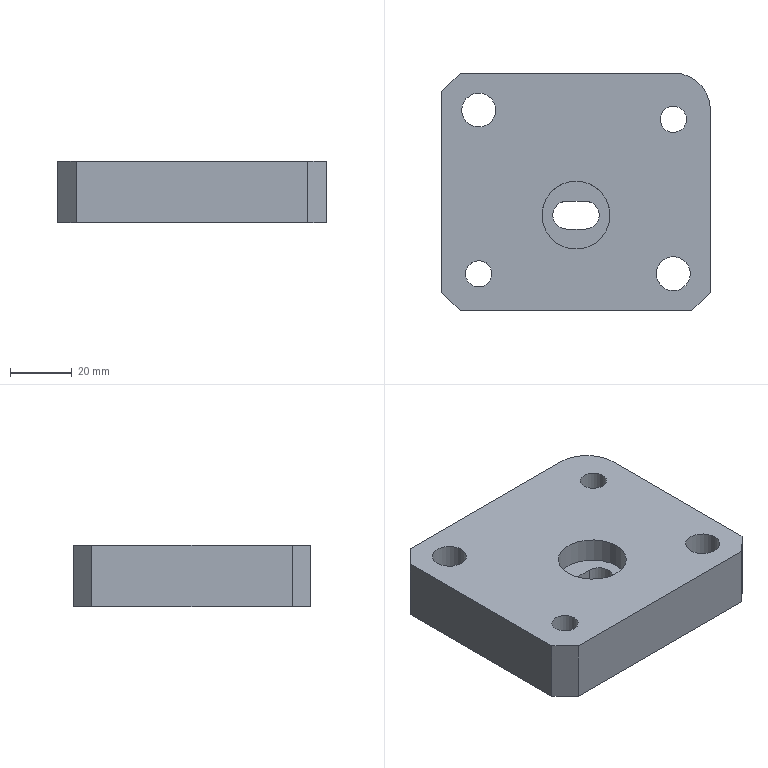Part | STEP file | lll_id3598_x_t | 1 solid | 28 faces | box 87 x 77 x 20 mm | volume 118043 mm3 | plane 16 | cylinder 12 | commonest cylinder face diameters 11 x4 8.5 x2 9.05 x2 17 x2 22 x1 24 x1
STEP:
#1=CARTESIAN_POINT('',(3550.234,-196.45,22.5));
#2=VERTEX_POINT('',#1);
#3=CARTESIAN_POINT('',(3555.734,-196.45,22.5));
#4=DIRECTION('',(0.,0.,-1.));
#5=DIRECTION('',(-1.,0.,0.));
#6=AXIS2_PLACEMENT_3D('',#3,#4,#5);
#7=CIRCLE('',#6,5.5);
#8=EDGE_CURVE('',#2,#2,#7,.T.);
#9=ORIENTED_EDGE('',*,*,#8,.T.);
#10=EDGE_LOOP('',(#9));
#11=FACE_BOUND('',#10,.T.);
#12=CARTESIAN_POINT('',(3543.734,-255.45,22.5));
#13=VERTEX_POINT('',#12);
#14=CARTESIAN_POINT('',(3543.734,-190.45,22.5));
#15=VERTEX_POINT('',#14);
#16=CARTESIAN_POINT('',(3543.734,-268.608,22.5));
#17=DIRECTION('',(0.,1.,0.));
#18=VECTOR('',#17,1.);
#19=LINE('',#16,#18);
#20=EDGE_CURVE('',#13,#15,#19,.T.);
#21=ORIENTED_EDGE('',*,*,#20,.F.);
#22=CARTESIAN_POINT('',(3549.734,-261.45,22.5));
#23=VERTEX_POINT('',#22);
#24=CARTESIAN_POINT('',(3727.771,-439.487,22.5));
#25=DIRECTION('',(0.7071,-0.7071,0.));
#26=VECTOR('',#25,1.);
#27=LINE('',#24,#26);
#28=EDGE_CURVE('',#13,#23,#27,.T.);
#29=ORIENTED_EDGE('',*,*,#28,.T.);
#30=CARTESIAN_POINT('',(3624.734,-261.45,22.5));
#31=VERTEX_POINT('',#30);
#32=CARTESIAN_POINT('',(3589.234,-261.45,22.5));
#33=DIRECTION('',(1.,0.,0.));
#34=VECTOR('',#33,1.);
#35=LINE('',#32,#34);
#36=EDGE_CURVE('',#23,#31,#35,.T.);
#37=ORIENTED_EDGE('',*,*,#36,.T.);
#38=CARTESIAN_POINT('',(3630.734,-255.45,22.5));
#39=VERTEX_POINT('',#38);
#40=CARTESIAN_POINT('',(3758.114,-128.07,22.5));
#41=DIRECTION('',(0.7071,0.7071,0.));
#42=VECTOR('',#41,1.);
#43=LINE('',#40,#42);
#44=EDGE_CURVE('',#31,#39,#43,.T.);
#45=ORIENTED_EDGE('',*,*,#44,.T.);
#46=CARTESIAN_POINT('',(3630.734,-196.45,22.5));
#47=VERTEX_POINT('',#46);
#48=CARTESIAN_POINT('',(3630.734,-239.45,22.5));
#49=DIRECTION('',(0.,1.,0.));
#50=VECTOR('',#49,1.);
#51=LINE('',#48,#50);
#52=EDGE_CURVE('',#39,#47,#51,.T.);
#53=ORIENTED_EDGE('',*,*,#52,.T.);
#54=CARTESIAN_POINT('',(3618.734,-184.45,22.5));
#55=VERTEX_POINT('',#54);
#56=CARTESIAN_POINT('',(3618.734,-196.45,22.5));
#57=DIRECTION('',(0.,0.,1.));
#58=DIRECTION('',(1.,0.,0.));
#59=AXIS2_PLACEMENT_3D('',#56,#57,#58);
#60=CIRCLE('',#59,12.);
#61=EDGE_CURVE('',#47,#55,#60,.T.);
#62=ORIENTED_EDGE('',*,*,#61,.T.);
#63=CARTESIAN_POINT('',(3549.734,-184.45,22.5));
#64=VERTEX_POINT('',#63);
#65=CARTESIAN_POINT('',(3589.234,-184.45,22.5));
#66=DIRECTION('',(-1.,0.,0.));
#67=VECTOR('',#66,1.);
#68=LINE('',#65,#67);
#69=EDGE_CURVE('',#55,#64,#68,.T.);
#70=ORIENTED_EDGE('',*,*,#69,.T.);
#71=CARTESIAN_POINT('',(3682.114,-52.07,22.5));
#72=DIRECTION('',(-0.7071,-0.7071,0.));
#73=VECTOR('',#72,1.);
#74=LINE('',#71,#73);
#75=EDGE_CURVE('',#64,#15,#74,.T.);
#76=ORIENTED_EDGE('',*,*,#75,.T.);
#77=EDGE_LOOP('',(#21,#29,#37,#45,#53,#62,#70,#76));
#78=FACE_BOUND('',#77,.T.);
#79=CARTESIAN_POINT('',(3613.234,-249.45,22.5));
#80=VERTEX_POINT('',#79);
#81=CARTESIAN_POINT('',(3618.734,-249.45,22.5));
#82=DIRECTION('',(0.,0.,-1.));
#83=DIRECTION('',(-1.,0.,0.));
#84=AXIS2_PLACEMENT_3D('',#81,#82,#83);
#85=CIRCLE('',#84,5.5);
#86=EDGE_CURVE('',#80,#80,#85,.T.);
#87=ORIENTED_EDGE('',*,*,#86,.T.);
#88=EDGE_LOOP('',(#87));
#89=FACE_BOUND('',#88,.T.);
#90=CARTESIAN_POINT('',(3551.484,-249.45,22.5));
#91=VERTEX_POINT('',#90);
#92=CARTESIAN_POINT('',(3555.734,-249.45,22.5));
#93=DIRECTION('',(0.,0.,-1.));
#94=DIRECTION('',(-1.,0.,0.));
#95=AXIS2_PLACEMENT_3D('',#92,#93,#94);
#96=CIRCLE('',#95,4.25);
#97=EDGE_CURVE('',#91,#91,#96,.T.);
#98=ORIENTED_EDGE('',*,*,#97,.T.);
#99=EDGE_LOOP('',(#98));
#100=FACE_BOUND('',#99,.T.);
#101=CARTESIAN_POINT('',(3614.484,-199.45,22.5));
#102=VERTEX_POINT('',#101);
#103=CARTESIAN_POINT('',(3618.734,-199.45,22.5));
#104=DIRECTION('',(0.,0.,-1.));
#105=DIRECTION('',(-1.,0.,0.));
#106=AXIS2_PLACEMENT_3D('',#103,#104,#105);
#107=CIRCLE('',#106,4.25);
#108=EDGE_CURVE('',#102,#102,#107,.T.);
#109=ORIENTED_EDGE('',*,*,#108,.T.);
#110=EDGE_LOOP('',(#109));
#111=FACE_BOUND('',#110,.T.);
#112=CARTESIAN_POINT('',(3576.234,-230.45,22.5));
#113=VERTEX_POINT('',#112);
#114=CARTESIAN_POINT('',(3587.234,-230.45,22.5));
#115=DIRECTION('',(0.,0.,-1.));
#116=DIRECTION('',(-1.,0.,0.));
#117=AXIS2_PLACEMENT_3D('',#114,#115,#116);
#118=CIRCLE('',#117,11.);
#119=EDGE_CURVE('',#113,#113,#118,.T.);
#120=ORIENTED_EDGE('',*,*,#119,.T.);
#121=EDGE_LOOP('',(#120));
#122=FACE_BOUND('',#121,.T.);
#123=CARTESIAN_POINT('',(3898.651,-268.608,22.5));
#124=DIRECTION('',(0.,0.,1.));
#125=DIRECTION('',(0.,-1.,0.));
#126=AXIS2_PLACEMENT_3D('',#123,#124,#125);
#127=PLANE('',#126);
#128=ADVANCED_FACE('',(#11,#78,#89,#100,#111,#122),#127,.T.);
#129=CARTESIAN_POINT('',(3590.234,-234.975,14.5));
#130=VERTEX_POINT('',#129);
#131=CARTESIAN_POINT('',(3590.234,-234.975,2.5));
#132=VERTEX_POINT('',#131);
#133=CARTESIAN_POINT('',(3590.234,-234.975,2.5));
#134=DIRECTION('',(0.000000008,0.,-1.));
#135=VECTOR('',#134,1.);
#136=LINE('',#133,#135);
#137=EDGE_CURVE('',#130,#132,#136,.T.);
#138=ORIENTED_EDGE('',*,*,#137,.F.);
#139=CARTESIAN_POINT('',(3590.234,-225.925,14.5));
#140=VERTEX_POINT('',#139);
#141=CARTESIAN_POINT('',(3590.234,-230.45,14.5));
#142=DIRECTION('',(0.,0.,1.));
#143=DIRECTION('',(1.,0.,0.));
#144=AXIS2_PLACEMENT_3D('',#141,#142,#143);
#145=CIRCLE('',#144,4.525);
#146=EDGE_CURVE('',#130,#140,#145,.T.);
#147=ORIENTED_EDGE('',*,*,#146,.T.);
#148=CARTESIAN_POINT('',(3590.234,-225.925,2.5));
#149=VERTEX_POINT('',#148);
#150=CARTESIAN_POINT('',(3590.234,-225.925,2.5));
#151=DIRECTION('',(0.000000008,0.,-1.));
#152=VECTOR('',#151,1.);
#153=LINE('',#150,#152);
#154=EDGE_CURVE('',#140,#149,#153,.T.);
#155=ORIENTED_EDGE('',*,*,#154,.T.);
#156=CARTESIAN_POINT('',(3590.234,-230.45,2.5));
#157=DIRECTION('',(0.,0.,-1.));
#158=DIRECTION('',(-1.,0.,0.));
#159=AXIS2_PLACEMENT_3D('',#156,#157,#158);
#160=CIRCLE('',#159,4.525);
#161=EDGE_CURVE('',#149,#132,#160,.T.);
#162=ORIENTED_EDGE('',*,*,#161,.T.);
#163=EDGE_LOOP('',(#138,#147,#155,#162));
#164=FACE_OUTER_BOUND('',#163,.T.);
#165=CARTESIAN_POINT('',(3590.234,-230.45,2.5));
#166=DIRECTION('',(-0.000000008,0.,1.));
#167=DIRECTION('',(-1.,0.,-0.000000008));
#168=AXIS2_PLACEMENT_3D('',#165,#166,#167);
#169=CYLINDRICAL_SURFACE('',#168,4.525);
#170=ADVANCED_FACE('',(#164),#169,.F.);
#171=ORIENTED_EDGE('',*,*,#154,.F.);
#172=CARTESIAN_POINT('',(3584.234,-225.925,14.5));
#173=VERTEX_POINT('',#172);
#174=CARTESIAN_POINT('',(3584.234,-225.925,14.5));
#175=DIRECTION('',(-1.,0.,0.));
#176=VECTOR('',#175,1.);
#177=LINE('',#174,#176);
#178=EDGE_CURVE('',#140,#173,#177,.T.);
#179=ORIENTED_EDGE('',*,*,#178,.T.);
#180=CARTESIAN_POINT('',(3584.234,-225.925,2.5));
#181=VERTEX_POINT('',#180);
#182=CARTESIAN_POINT('',(3584.234,-225.925,2.5));
#183=DIRECTION('',(0.000000008,0.,-1.));
#184=VECTOR('',#183,1.);
#185=LINE('',#182,#184);
#186=EDGE_CURVE('',#173,#181,#185,.T.);
#187=ORIENTED_EDGE('',*,*,#186,.T.);
#188=CARTESIAN_POINT('',(3898.651,-225.925,2.5));
#189=DIRECTION('',(1.,0.,0.));
#190=VECTOR('',#189,1.);
#191=LINE('',#188,#190);
#192=EDGE_CURVE('',#181,#149,#191,.T.);
#193=ORIENTED_EDGE('',*,*,#192,.T.);
#194=EDGE_LOOP('',(#171,#179,#187,#193));
#195=FACE_OUTER_BOUND('',#194,.T.);
#196=CARTESIAN_POINT('',(3584.234,-225.925,2.5));
#197=DIRECTION('',(0.,-1.,0.));
#198=DIRECTION('',(1.,0.,0.000000008));
#199=AXIS2_PLACEMENT_3D('',#196,#197,#198);
#200=PLANE('',#199);
#201=ADVANCED_FACE('',(#195),#200,.T.);
#202=ORIENTED_EDGE('',*,*,#186,.F.);
#203=CARTESIAN_POINT('',(3584.234,-234.975,14.5));
#204=VERTEX_POINT('',#203);
#205=CARTESIAN_POINT('',(3584.234,-230.45,14.5));
#206=DIRECTION('',(0.,0.,1.));
#207=DIRECTION('',(1.,0.,0.));
#208=AXIS2_PLACEMENT_3D('',#205,#206,#207);
#209=CIRCLE('',#208,4.525);
#210=EDGE_CURVE('',#173,#204,#209,.T.);
#211=ORIENTED_EDGE('',*,*,#210,.T.);
#212=CARTESIAN_POINT('',(3584.234,-234.975,2.5));
#213=VERTEX_POINT('',#212);
#214=CARTESIAN_POINT('',(3584.234,-234.975,2.5));
#215=DIRECTION('',(0.000000008,0.,-1.));
#216=VECTOR('',#215,1.);
#217=LINE('',#214,#216);
#218=EDGE_CURVE('',#204,#213,#217,.T.);
#219=ORIENTED_EDGE('',*,*,#218,.T.);
#220=CARTESIAN_POINT('',(3584.234,-230.45,2.5));
#221=DIRECTION('',(0.,0.,-1.));
#222=DIRECTION('',(-1.,0.,0.));
#223=AXIS2_PLACEMENT_3D('',#220,#221,#222);
#224=CIRCLE('',#223,4.525);
#225=EDGE_CURVE('',#213,#181,#224,.T.);
#226=ORIENTED_EDGE('',*,*,#225,.T.);
#227=EDGE_LOOP('',(#202,#211,#219,#226));
#228=FACE_OUTER_BOUND('',#227,.T.);
#229=CARTESIAN_POINT('',(3584.234,-230.45,2.5));
#230=DIRECTION('',(-0.000000008,0.,1.));
#231=DIRECTION('',(-1.,0.,-0.000000008));
#232=AXIS2_PLACEMENT_3D('',#229,#230,#231);
#233=CYLINDRICAL_SURFACE('',#232,4.525);
#234=ADVANCED_FACE('',(#228),#233,.F.);
#235=ORIENTED_EDGE('',*,*,#218,.F.);
#236=CARTESIAN_POINT('',(3584.234,-234.975,14.5));
#237=DIRECTION('',(1.,0.,0.));
#238=VECTOR('',#237,1.);
#239=LINE('',#236,#238);
#240=EDGE_CURVE('',#204,#130,#239,.T.);
#241=ORIENTED_EDGE('',*,*,#240,.T.);
#242=ORIENTED_EDGE('',*,*,#137,.T.);
#243=CARTESIAN_POINT('',(3898.651,-234.975,2.5));
#244=DIRECTION('',(-1.,0.,0.));
#245=VECTOR('',#244,1.);
#246=LINE('',#243,#245);
#247=EDGE_CURVE('',#132,#213,#246,.T.);
#248=ORIENTED_EDGE('',*,*,#247,.T.);
#249=EDGE_LOOP('',(#235,#241,#242,#248));
#250=FACE_OUTER_BOUND('',#249,.T.);
#251=CARTESIAN_POINT('',(3584.234,-234.975,2.5));
#252=DIRECTION('',(0.,-1.,0.));
#253=DIRECTION('',(1.,0.,0.000000008));
#254=AXIS2_PLACEMENT_3D('',#251,#252,#253);
#255=PLANE('',#254);
#256=ADVANCED_FACE('',(#250),#255,.F.);
#257=ORIENTED_EDGE('',*,*,#161,.F.);
#258=ORIENTED_EDGE('',*,*,#192,.F.);
#259=ORIENTED_EDGE('',*,*,#225,.F.);
#260=ORIENTED_EDGE('',*,*,#247,.F.);
#261=EDGE_LOOP('',(#257,#258,#259,#260));
#262=FACE_BOUND('',#261,.T.);
#263=CARTESIAN_POINT('',(3550.234,-249.45,2.5));
#264=VERTEX_POINT('',#263);
#265=CARTESIAN_POINT('',(3555.734,-249.45,2.5));
#266=DIRECTION('',(0.,0.,-1.));
#267=DIRECTION('',(-1.,0.,0.));
#268=AXIS2_PLACEMENT_3D('',#265,#266,#267);
#269=CIRCLE('',#268,5.5);
#270=EDGE_CURVE('',#264,#264,#269,.T.);
#271=ORIENTED_EDGE('',*,*,#270,.F.);
#272=EDGE_LOOP('',(#271));
#273=FACE_BOUND('',#272,.T.);
#274=CARTESIAN_POINT('',(3610.234,-249.45,2.5));
#275=VERTEX_POINT('',#274);
#276=CARTESIAN_POINT('',(3618.734,-249.45,2.5));
#277=DIRECTION('',(0.,0.,1.));
#278=DIRECTION('',(-1.,0.,0.));
#279=AXIS2_PLACEMENT_3D('',#276,#277,#278);
#280=CIRCLE('',#279,8.5);
#281=EDGE_CURVE('',#275,#275,#280,.T.);
#282=ORIENTED_EDGE('',*,*,#281,.T.);
#283=EDGE_LOOP('',(#282));
#284=FACE_BOUND('',#283,.T.);
#285=CARTESIAN_POINT('',(3624.734,-261.45,2.5));
#286=VERTEX_POINT('',#285);
#287=CARTESIAN_POINT('',(3549.734,-261.45,2.5));
#288=VERTEX_POINT('',#287);
#289=CARTESIAN_POINT('',(3589.234,-261.45,2.5));
#290=DIRECTION('',(-1.,0.,0.));
#291=VECTOR('',#290,1.);
#292=LINE('',#289,#291);
#293=EDGE_CURVE('',#286,#288,#292,.T.);
#294=ORIENTED_EDGE('',*,*,#293,.T.);
#295=CARTESIAN_POINT('',(3543.734,-255.45,2.5));
#296=VERTEX_POINT('',#295);
#297=CARTESIAN_POINT('',(3543.734,-255.45,2.5));
#298=DIRECTION('',(-0.7071,0.7071,0.));
#299=VECTOR('',#298,1.);
#300=LINE('',#297,#299);
#301=EDGE_CURVE('',#288,#296,#300,.T.);
#302=ORIENTED_EDGE('',*,*,#301,.T.);
#303=CARTESIAN_POINT('',(3543.734,-190.45,2.5));
#304=VERTEX_POINT('',#303);
#305=CARTESIAN_POINT('',(3543.734,-268.608,2.5));
#306=DIRECTION('',(0.,-1.,0.));
#307=VECTOR('',#306,1.);
#308=LINE('',#305,#307);
#309=EDGE_CURVE('',#304,#296,#308,.T.);
#310=ORIENTED_EDGE('',*,*,#309,.F.);
#311=CARTESIAN_POINT('',(3549.734,-184.45,2.5));
#312=VERTEX_POINT('',#311);
#313=CARTESIAN_POINT('',(3543.734,-190.45,2.5));
#314=DIRECTION('',(0.7071,0.7071,0.));
#315=VECTOR('',#314,1.);
#316=LINE('',#313,#315);
#317=EDGE_CURVE('',#304,#312,#316,.T.);
#318=ORIENTED_EDGE('',*,*,#317,.T.);
#319=CARTESIAN_POINT('',(3618.734,-184.45,2.5));
#320=VERTEX_POINT('',#319);
#321=CARTESIAN_POINT('',(3589.234,-184.45,2.5));
#322=DIRECTION('',(1.,0.,0.));
#323=VECTOR('',#322,1.);
#324=LINE('',#321,#323);
#325=EDGE_CURVE('',#312,#320,#324,.T.);
#326=ORIENTED_EDGE('',*,*,#325,.T.);
#327=CARTESIAN_POINT('',(3630.734,-196.45,2.5));
#328=VERTEX_POINT('',#327);
#329=CARTESIAN_POINT('',(3618.734,-196.45,2.5));
#330=DIRECTION('',(0.,0.,-1.));
#331=DIRECTION('',(1.,0.,0.));
#332=AXIS2_PLACEMENT_3D('',#329,#330,#331);
#333=CIRCLE('',#332,12.);
#334=EDGE_CURVE('',#320,#328,#333,.T.);
#335=ORIENTED_EDGE('',*,*,#334,.T.);
#336=CARTESIAN_POINT('',(3630.734,-255.45,2.5));
#337=VERTEX_POINT('',#336);
#338=CARTESIAN_POINT('',(3630.734,-239.45,2.5));
#339=DIRECTION('',(0.,-1.,0.));
#340=VECTOR('',#339,1.);
#341=LINE('',#338,#340);
#342=EDGE_CURVE('',#328,#337,#341,.T.);
#343=ORIENTED_EDGE('',*,*,#342,.T.);
#344=CARTESIAN_POINT('',(3624.734,-261.45,2.5));
#345=DIRECTION('',(-0.7071,-0.7071,0.));
#346=VECTOR('',#345,1.);
#347=LINE('',#344,#346);
#348=EDGE_CURVE('',#337,#286,#347,.T.);
#349=ORIENTED_EDGE('',*,*,#348,.T.);
#350=EDGE_LOOP('',(#294,#302,#310,#318,#326,#335,#343,#349));
#351=FACE_BOUND('',#350,.T.);
#352=CARTESIAN_POINT('',(3547.234,-196.45,2.5));
#353=VERTEX_POINT('',#352);
#354=CARTESIAN_POINT('',(3555.734,-196.45,2.5));
#355=DIRECTION('',(0.,0.,-1.));
#356=DIRECTION('',(-1.,0.,0.));
#357=AXIS2_PLACEMENT_3D('',#354,#355,#356);
#358=CIRCLE('',#357,8.5);
#359=EDGE_CURVE('',#353,#353,#358,.T.);
#360=ORIENTED_EDGE('',*,*,#359,.F.);
#361=EDGE_LOOP('',(#360));
#362=FACE_BOUND('',#361,.T.);
#363=CARTESIAN_POINT('',(3613.234,-199.45,2.5));
#364=VERTEX_POINT('',#363);
#365=CARTESIAN_POINT('',(3618.734,-199.45,2.5));
#366=DIRECTION('',(0.,0.,1.));
#367=DIRECTION('',(-1.,0.,0.));
#368=AXIS2_PLACEMENT_3D('',#365,#366,#367);
#369=CIRCLE('',#368,5.5);
#370=EDGE_CURVE('',#364,#364,#369,.T.);
#371=ORIENTED_EDGE('',*,*,#370,.T.);
#372=EDGE_LOOP('',(#371));
#373=FACE_BOUND('',#372,.T.);
#374=CARTESIAN_POINT('',(3898.651,-268.608,2.5));
#375=DIRECTION('',(0.,0.,1.));
#376=DIRECTION('',(0.,-1.,0.));
#377=AXIS2_PLACEMENT_3D('',#374,#375,#376);
#378=PLANE('',#377);
#379=ADVANCED_FACE('',(#262,#273,#284,#351,#362,#373),#378,.F.);
#380=CARTESIAN_POINT('',(3551.484,-249.45,9.5));
#381=VERTEX_POINT('',#380);
#382=CARTESIAN_POINT('',(3555.734,-249.45,9.5));
#383=DIRECTION('',(0.,0.,1.));
#384=DIRECTION('',(-1.,0.,0.));
#385=AXIS2_PLACEMENT_3D('',#382,#383,#384);
#386=CIRCLE('',#385,4.25);
#387=EDGE_CURVE('',#381,#381,#386,.T.);
#388=ORIENTED_EDGE('',*,*,#387,.T.);
#389=EDGE_LOOP('',(#388));
#390=FACE_BOUND('',#389,.T.);
#391=CARTESIAN_POINT('',(3550.234,-249.45,9.5));
#392=VERTEX_POINT('',#391);
#393=CARTESIAN_POINT('',(3555.734,-249.45,9.5));
#394=DIRECTION('',(0.,0.,1.));
#395=DIRECTION('',(-1.,0.,0.));
#396=AXIS2_PLACEMENT_3D('',#393,#394,#395);
#397=CIRCLE('',#396,5.5);
#398=EDGE_CURVE('',#392,#392,#397,.T.);
#399=ORIENTED_EDGE('',*,*,#398,.F.);
#400=EDGE_LOOP('',(#399));
#401=FACE_BOUND('',#400,.T.);
#402=CARTESIAN_POINT('',(3555.734,-249.45,9.5));
#403=DIRECTION('',(0.,0.,1.));
#404=DIRECTION('',(-1.,0.,0.));
#405=AXIS2_PLACEMENT_3D('',#402,#403,#404);
#406=PLANE('',#405);
#407=ADVANCED_FACE('',(#390,#401),#406,.F.);
#408=CARTESIAN_POINT('',(3613.234,-249.45,14.5));
#409=VERTEX_POINT('',#408);
#410=CARTESIAN_POINT('',(3618.734,-249.45,14.5));
#411=DIRECTION('',(0.,0.,-1.));
#412=DIRECTION('',(-1.,0.,0.));
#413=AXIS2_PLACEMENT_3D('',#410,#411,#412);
#414=CIRCLE('',#413,5.5);
#415=EDGE_CURVE('',#409,#409,#414,.T.);
#416=ORIENTED_EDGE('',*,*,#415,.F.);
#417=EDGE_LOOP('',(#416));
#418=FACE_BOUND('',#417,.T.);
#419=CARTESIAN_POINT('',(3610.234,-249.45,14.5));
#420=VERTEX_POINT('',#419);
#421=CARTESIAN_POINT('',(3618.734,-249.45,14.5));
#422=DIRECTION('',(0.,0.,-1.));
#423=DIRECTION('',(-1.,0.,0.));
#424=AXIS2_PLACEMENT_3D('',#421,#422,#423);
#425=CIRCLE('',#424,8.5);
#426=EDGE_CURVE('',#420,#420,#425,.T.);
#427=ORIENTED_EDGE('',*,*,#426,.T.);
#428=EDGE_LOOP('',(#427));
#429=FACE_BOUND('',#428,.T.);
#430=CARTESIAN_POINT('',(3618.734,-249.45,14.5));
#431=DIRECTION('',(0.,0.,1.));
#432=DIRECTION('',(0.,1.,0.));
#433=AXIS2_PLACEMENT_3D('',#430,#431,#432);
#434=PLANE('',#433);
#435=ADVANCED_FACE('',(#418,#429),#434,.F.);
#436=CARTESIAN_POINT('',(3550.234,-196.45,14.5));
#437=VERTEX_POINT('',#436);
#438=CARTESIAN_POINT('',(3555.734,-196.45,14.5));
#439=DIRECTION('',(0.,0.,1.));
#440=DIRECTION('',(-1.,0.,0.));
#441=AXIS2_PLACEMENT_3D('',#438,#439,#440);
#442=CIRCLE('',#441,5.5);
#443=EDGE_CURVE('',#437,#437,#442,.T.);
#444=ORIENTED_EDGE('',*,*,#443,.T.);
#445=EDGE_LOOP('',(#444));
#446=FACE_BOUND('',#445,.T.);
#447=CARTESIAN_POINT('',(3547.234,-196.45,14.5));
#448=VERTEX_POINT('',#447);
#449=CARTESIAN_POINT('',(3555.734,-196.45,14.5));
#450=DIRECTION('',(0.,0.,1.));
#451=DIRECTION('',(-1.,0.,0.));
#452=AXIS2_PLACEMENT_3D('',#449,#450,#451);
#453=CIRCLE('',#452,8.5);
#454=EDGE_CURVE('',#448,#448,#453,.T.);
#455=ORIENTED_EDGE('',*,*,#454,.F.);
#456=EDGE_LOOP('',(#455));
#457=FACE_BOUND('',#456,.T.);
#458=CARTESIAN_POINT('',(3555.734,-196.45,14.5));
#459=DIRECTION('',(0.,0.,1.));
#460=DIRECTION('',(0.,-1.,0.));
#461=AXIS2_PLACEMENT_3D('',#458,#459,#460);
#462=PLANE('',#461);
#463=ADVANCED_FACE('',(#446,#457),#462,.F.);
#464=ORIENTED_EDGE('',*,*,#8,.F.);
#465=EDGE_LOOP('',(#464));
#466=FACE_BOUND('',#465,.T.);
#467=ORIENTED_EDGE('',*,*,#443,.F.);
#468=EDGE_LOOP('',(#467));
#469=FACE_BOUND('',#468,.T.);
#470=CARTESIAN_POINT('',(3555.734,-196.45,97.5));
#471=DIRECTION('',(0.,0.,1.));
#472=DIRECTION('',(0.,-1.,0.));
#473=AXIS2_PLACEMENT_3D('',#470,#471,#472);
#474=CYLINDRICAL_SURFACE('',#473,5.5);
#475=ADVANCED_FACE('',(#466,#469),#474,.F.);
#476=ORIENTED_EDGE('',*,*,#398,.T.);
#477=EDGE_LOOP('',(#476));
#478=FACE_BOUND('',#477,.T.);
#479=ORIENTED_EDGE('',*,*,#270,.T.);
#480=EDGE_LOOP('',(#479));
#481=FACE_BOUND('',#480,.T.);
#482=CARTESIAN_POINT('',(3555.734,-249.45,-2.5));
#483=DIRECTION('',(0.,0.,1.));
#484=DIRECTION('',(-1.,0.,0.));
#485=AXIS2_PLACEMENT_3D('',#482,#483,#484);
#486=CYLINDRICAL_SURFACE('',#485,5.5);
#487=ADVANCED_FACE('',(#478,#481),#486,.F.);
#488=ORIENTED_EDGE('',*,*,#426,.F.);
#489=EDGE_LOOP('',(#488));
#490=FACE_BOUND('',#489,.T.);
#491=ORIENTED_EDGE('',*,*,#281,.F.);
#492=EDGE_LOOP('',(#491));
#493=FACE_BOUND('',#492,.T.);
#494=CARTESIAN_POINT('',(3618.734,-249.45,-2.5));
#495=DIRECTION('',(0.,0.,1.));
#496=DIRECTION('',(0.,1.,0.));
#497=AXIS2_PLACEMENT_3D('',#494,#495,#496);
#498=CYLINDRICAL_SURFACE('',#497,8.5);
#499=ADVANCED_FACE('',(#490,#493),#498,.F.);
#500=ORIENTED_EDGE('',*,*,#52,.F.);
#501=CARTESIAN_POINT('',(3630.734,-255.45,-81.5));
#502=DIRECTION('',(0.,0.,-1.));
#503=VECTOR('',#502,1.);
#504=LINE('',#501,#503);
#505=EDGE_CURVE('',#39,#337,#504,.T.);
#506=ORIENTED_EDGE('',*,*,#505,.T.);
#507=ORIENTED_EDGE('',*,*,#342,.F.);
#508=CARTESIAN_POINT('',(3630.734,-196.45,-81.5));
#509=DIRECTION('',(0.,0.,1.));
#510=VECTOR('',#509,1.);
#511=LINE('',#508,#510);
#512=EDGE_CURVE('',#328,#47,#511,.T.);
#513=ORIENTED_EDGE('',*,*,#512,.T.);
#514=EDGE_LOOP('',(#500,#506,#507,#513));
#515=FACE_OUTER_BOUND('',#514,.T.);
#516=CARTESIAN_POINT('',(3630.734,-239.45,-81.5));
#517=DIRECTION('',(1.,0.,0.));
#518=DIRECTION('',(0.,0.,-1.));
#519=AXIS2_PLACEMENT_3D('',#516,#517,#518);
#520=PLANE('',#519);
#521=ADVANCED_FACE('',(#515),#520,.T.);
#522=ORIENTED_EDGE('',*,*,#36,.F.);
#523=CARTESIAN_POINT('',(3549.734,-261.45,-81.5));
#524=DIRECTION('',(0.,0.,-1.));
#525=VECTOR('',#524,1.);
#526=LINE('',#523,#525);
#527=EDGE_CURVE('',#23,#288,#526,.T.);
#528=ORIENTED_EDGE('',*,*,#527,.T.);
#529=ORIENTED_EDGE('',*,*,#293,.F.);
#530=CARTESIAN_POINT('',(3624.734,-261.45,-81.5));
#531=DIRECTION('',(0.,0.,1.));
#532=VECTOR('',#531,1.);
#533=LINE('',#530,#532);
#534=EDGE_CURVE('',#286,#31,#533,.T.);
#535=ORIENTED_EDGE('',*,*,#534,.T.);
#536=EDGE_LOOP('',(#522,#528,#529,#535));
#537=FACE_OUTER_BOUND('',#536,.T.);
#538=CARTESIAN_POINT('',(3589.234,-261.45,-81.5));
#539=DIRECTION('',(0.,-1.,0.));
#540=DIRECTION('',(0.,0.,-1.));
#541=AXIS2_PLACEMENT_3D('',#538,#539,#540);
#542=PLANE('',#541);
#543=ADVANCED_FACE('',(#537),#542,.T.);
#544=ORIENTED_EDGE('',*,*,#309,.T.);
#545=CARTESIAN_POINT('',(3543.734,-255.45,13.5));
#546=DIRECTION('',(0.,0.,1.));
#547=VECTOR('',#546,1.);
#548=LINE('',#545,#547);
#549=EDGE_CURVE('',#296,#13,#548,.T.);
#550=ORIENTED_EDGE('',*,*,#549,.T.);
#551=ORIENTED_EDGE('',*,*,#20,.T.);
#552=CARTESIAN_POINT('',(3543.734,-190.45,13.5));
#553=DIRECTION('',(0.,0.,-1.));
#554=VECTOR('',#553,1.);
#555=LINE('',#552,#554);
#556=EDGE_CURVE('',#15,#304,#555,.T.);
#557=ORIENTED_EDGE('',*,*,#556,.T.);
#558=EDGE_LOOP('',(#544,#550,#551,#557));
#559=FACE_OUTER_BOUND('',#558,.T.);
#560=CARTESIAN_POINT('',(3543.734,-239.45,13.5));
#561=DIRECTION('',(-1.,0.,0.));
#562=DIRECTION('',(0.,0.,1.));
#563=AXIS2_PLACEMENT_3D('',#560,#561,#562);
#564=PLANE('',#563);
#565=ADVANCED_FACE('',(#559),#564,.T.);
#566=ORIENTED_EDGE('',*,*,#325,.F.);
#567=CARTESIAN_POINT('',(3549.734,-184.45,-81.5));
#568=DIRECTION('',(0.,0.,1.));
#569=VECTOR('',#568,1.);
#570=LINE('',#567,#569);
#571=EDGE_CURVE('',#312,#64,#570,.T.);
#572=ORIENTED_EDGE('',*,*,#571,.T.);
#573=ORIENTED_EDGE('',*,*,#69,.F.);
#574=CARTESIAN_POINT('',(3618.734,-184.45,-81.5));
#575=DIRECTION('',(0.,0.,-1.));
#576=VECTOR('',#575,1.);
#577=LINE('',#574,#576);
#578=EDGE_CURVE('',#55,#320,#577,.T.);
#579=ORIENTED_EDGE('',*,*,#578,.T.);
#580=EDGE_LOOP('',(#566,#572,#573,#579));
#581=FACE_OUTER_BOUND('',#580,.T.);
#582=CARTESIAN_POINT('',(3589.234,-184.45,-81.5));
#583=DIRECTION('',(0.,1.,0.));
#584=DIRECTION('',(0.,0.,1.));
#585=AXIS2_PLACEMENT_3D('',#582,#583,#584);
#586=PLANE('',#585);
#587=ADVANCED_FACE('',(#581),#586,.T.);
#588=ORIENTED_EDGE('',*,*,#454,.T.);
#589=EDGE_LOOP('',(#588));
#590=FACE_BOUND('',#589,.T.);
#591=ORIENTED_EDGE('',*,*,#359,.T.);
#592=EDGE_LOOP('',(#591));
#593=FACE_BOUND('',#592,.T.);
#594=CARTESIAN_POINT('',(3555.734,-196.45,-2.5));
#595=DIRECTION('',(0.,0.,1.));
#596=DIRECTION('',(0.,-1.,0.));
#597=AXIS2_PLACEMENT_3D('',#594,#595,#596);
#598=CYLINDRICAL_SURFACE('',#597,8.5);
#599=ADVANCED_FACE('',(#590,#593),#598,.F.);
#600=ORIENTED_EDGE('',*,*,#86,.F.);
#601=EDGE_LOOP('',(#600));
#602=FACE_BOUND('',#601,.T.);
#603=ORIENTED_EDGE('',*,*,#415,.T.);
#604=EDGE_LOOP('',(#603));
#605=FACE_BOUND('',#604,.T.);
#606=CARTESIAN_POINT('',(3618.734,-249.45,97.5));
#607=DIRECTION('',(0.,0.,1.));
#608=DIRECTION('',(0.,1.,0.));
#609=AXIS2_PLACEMENT_3D('',#606,#607,#608);
#610=CYLINDRICAL_SURFACE('',#609,5.5);
#611=ADVANCED_FACE('',(#602,#605),#610,.F.);
#612=ORIENTED_EDGE('',*,*,#97,.F.);
#613=EDGE_LOOP('',(#612));
#614=FACE_BOUND('',#613,.T.);
#615=ORIENTED_EDGE('',*,*,#387,.F.);
#616=EDGE_LOOP('',(#615));
#617=FACE_BOUND('',#616,.T.);
#618=CARTESIAN_POINT('',(3555.734,-249.45,97.5));
#619=DIRECTION('',(0.,0.,1.));
#620=DIRECTION('',(-1.,0.,0.));
#621=AXIS2_PLACEMENT_3D('',#618,#619,#620);
#622=CYLINDRICAL_SURFACE('',#621,4.25);
#623=ADVANCED_FACE('',(#614,#617),#622,.F.);
#624=ORIENTED_EDGE('',*,*,#108,.F.);
#625=EDGE_LOOP('',(#624));
#626=FACE_BOUND('',#625,.T.);
#627=CARTESIAN_POINT('',(3614.484,-199.45,9.5));
#628=VERTEX_POINT('',#627);
#629=CARTESIAN_POINT('',(3618.734,-199.45,9.5));
#630=DIRECTION('',(0.,0.,1.));
#631=DIRECTION('',(-1.,0.,0.));
#632=AXIS2_PLACEMENT_3D('',#629,#630,#631);
#633=CIRCLE('',#632,4.25);
#634=EDGE_CURVE('',#628,#628,#633,.T.);
#635=ORIENTED_EDGE('',*,*,#634,.F.);
#636=EDGE_LOOP('',(#635));
#637=FACE_BOUND('',#636,.T.);
#638=CARTESIAN_POINT('',(3618.734,-199.45,97.5));
#639=DIRECTION('',(0.,0.,1.));
#640=DIRECTION('',(1.,0.,0.));
#641=AXIS2_PLACEMENT_3D('',#638,#639,#640);
#642=CYLINDRICAL_SURFACE('',#641,4.25);
#643=ADVANCED_FACE('',(#626,#637),#642,.F.);
#644=ORIENTED_EDGE('',*,*,#634,.T.);
#645=EDGE_LOOP('',(#644));
#646=FACE_BOUND('',#645,.T.);
#647=CARTESIAN_POINT('',(3613.234,-199.45,9.5));
#648=VERTEX_POINT('',#647);
#649=CARTESIAN_POINT('',(3618.734,-199.45,9.5));
#650=DIRECTION('',(0.,0.,1.));
#651=DIRECTION('',(-1.,0.,0.));
#652=AXIS2_PLACEMENT_3D('',#649,#650,#651);
#653=CIRCLE('',#652,5.5);
#654=EDGE_CURVE('',#648,#648,#653,.T.);
#655=ORIENTED_EDGE('',*,*,#654,.F.);
#656=EDGE_LOOP('',(#655));
#657=FACE_BOUND('',#656,.T.);
#658=CARTESIAN_POINT('',(3618.734,-199.45,9.5));
#659=DIRECTION('',(0.,0.,1.));
#660=DIRECTION('',(1.,0.,0.));
#661=AXIS2_PLACEMENT_3D('',#658,#659,#660);
#662=PLANE('',#661);
#663=ADVANCED_FACE('',(#646,#657),#662,.F.);
#664=ORIENTED_EDGE('',*,*,#654,.T.);
#665=EDGE_LOOP('',(#664));
#666=FACE_BOUND('',#665,.T.);
#667=ORIENTED_EDGE('',*,*,#370,.F.);
#668=EDGE_LOOP('',(#667));
#669=FACE_BOUND('',#668,.T.);
#670=CARTESIAN_POINT('',(3618.734,-199.45,-2.5));
#671=DIRECTION('',(0.,0.,1.));
#672=DIRECTION('',(1.,0.,0.));
#673=AXIS2_PLACEMENT_3D('',#670,#671,#672);
#674=CYLINDRICAL_SURFACE('',#673,5.5);
#675=ADVANCED_FACE('',(#666,#669),#674,.F.);
#676=CARTESIAN_POINT('',(3598.234,-230.45,14.5));
#677=VERTEX_POINT('',#676);
#678=CARTESIAN_POINT('',(3587.234,-230.45,14.5));
#679=DIRECTION('',(0.,0.,1.));
#680=DIRECTION('',(1.,0.,0.));
#681=AXIS2_PLACEMENT_3D('',#678,#679,#680);
#682=CIRCLE('',#681,11.);
#683=EDGE_CURVE('',#677,#677,#682,.T.);
#684=ORIENTED_EDGE('',*,*,#683,.T.);
#685=EDGE_LOOP('',(#684));
#686=FACE_BOUND('',#685,.T.);
#687=ORIENTED_EDGE('',*,*,#240,.F.);
#688=ORIENTED_EDGE('',*,*,#210,.F.);
#689=ORIENTED_EDGE('',*,*,#178,.F.);
#690=ORIENTED_EDGE('',*,*,#146,.F.);
#691=EDGE_LOOP('',(#687,#688,#689,#690));
#692=FACE_BOUND('',#691,.T.);
#693=CARTESIAN_POINT('',(3587.234,-230.45,14.5));
#694=DIRECTION('',(0.,0.,-1.));
#695=DIRECTION('',(1.,0.,0.));
#696=AXIS2_PLACEMENT_3D('',#693,#694,#695);
#697=PLANE('',#696);
#698=ADVANCED_FACE('',(#686,#692),#697,.F.);
#699=ORIENTED_EDGE('',*,*,#119,.F.);
#700=EDGE_LOOP('',(#699));
#701=FACE_BOUND('',#700,.T.);
#702=ORIENTED_EDGE('',*,*,#683,.F.);
#703=EDGE_LOOP('',(#702));
#704=FACE_BOUND('',#703,.T.);
#705=CARTESIAN_POINT('',(3587.234,-230.45,14.5));
#706=DIRECTION('',(0.,0.,1.));
#707=DIRECTION('',(-1.,0.,0.));
#708=AXIS2_PLACEMENT_3D('',#705,#706,#707);
#709=CYLINDRICAL_SURFACE('',#708,11.);
#710=ADVANCED_FACE('',(#701,#704),#709,.F.);
#711=ORIENTED_EDGE('',*,*,#334,.F.);
#712=ORIENTED_EDGE('',*,*,#578,.F.);
#713=ORIENTED_EDGE('',*,*,#61,.F.);
#714=ORIENTED_EDGE('',*,*,#512,.F.);
#715=EDGE_LOOP('',(#711,#712,#713,#714));
#716=FACE_OUTER_BOUND('',#715,.T.);
#717=CARTESIAN_POINT('',(3618.734,-196.45,-81.5));
#718=DIRECTION('',(0.,0.,-1.));
#719=DIRECTION('',(1.,0.,0.));
#720=AXIS2_PLACEMENT_3D('',#717,#718,#719);
#721=CYLINDRICAL_SURFACE('',#720,12.);
#722=ADVANCED_FACE('',(#716),#721,.T.);
#723=ORIENTED_EDGE('',*,*,#301,.F.);
#724=ORIENTED_EDGE('',*,*,#527,.F.);
#725=ORIENTED_EDGE('',*,*,#28,.F.);
#726=ORIENTED_EDGE('',*,*,#549,.F.);
#727=EDGE_LOOP('',(#723,#724,#725,#726));
#728=FACE_OUTER_BOUND('',#727,.T.);
#729=CARTESIAN_POINT('',(3543.734,-255.45,13.5));
#730=DIRECTION('',(0.7071,0.7071,0.));
#731=DIRECTION('',(0.,0.,-1.));
#732=AXIS2_PLACEMENT_3D('',#729,#730,#731);
#733=PLANE('',#732);
#734=ADVANCED_FACE('',(#728),#733,.F.);
#735=ORIENTED_EDGE('',*,*,#75,.F.);
#736=ORIENTED_EDGE('',*,*,#571,.F.);
#737=ORIENTED_EDGE('',*,*,#317,.F.);
#738=ORIENTED_EDGE('',*,*,#556,.F.);
#739=EDGE_LOOP('',(#735,#736,#737,#738));
#740=FACE_OUTER_BOUND('',#739,.T.);
#741=CARTESIAN_POINT('',(3543.734,-190.45,13.5));
#742=DIRECTION('',(0.7071,-0.7071,0.));
#743=DIRECTION('',(0.,0.,1.));
#744=AXIS2_PLACEMENT_3D('',#741,#742,#743);
#745=PLANE('',#744);
#746=ADVANCED_FACE('',(#740),#745,.F.);
#747=ORIENTED_EDGE('',*,*,#348,.F.);
#748=ORIENTED_EDGE('',*,*,#505,.F.);
#749=ORIENTED_EDGE('',*,*,#44,.F.);
#750=ORIENTED_EDGE('',*,*,#534,.F.);
#751=EDGE_LOOP('',(#747,#748,#749,#750));
#752=FACE_OUTER_BOUND('',#751,.T.);
#753=CARTESIAN_POINT('',(3624.734,-261.45,-81.5));
#754=DIRECTION('',(-0.7071,0.7071,0.));
#755=DIRECTION('',(0.,0.,-1.));
#756=AXIS2_PLACEMENT_3D('',#753,#754,#755);
#757=PLANE('',#756);
#758=ADVANCED_FACE('',(#752),#757,.F.);
#759=CLOSED_SHELL('',(#128,#170,#201,#234,#256,#379,#407,#435,#463,#475,#487,#499,#521,#543,#565,#587,#599,#611,#623,#643,#663,#675,#698,#710,#722,#734,#746,#758));
#760=MANIFOLD_SOLID_BREP('',#759);
#761=(LENGTH_UNIT()NAMED_UNIT(*)SI_UNIT(.MILLI.,.METRE.));
#762=UNCERTAINTY_MEASURE_WITH_UNIT(LENGTH_MEASURE(0.00002),#761,'','');
#763=(NAMED_UNIT(*)PLANE_ANGLE_UNIT()SI_UNIT($,.RADIAN.));
#764=PLANE_ANGLE_MEASURE_WITH_UNIT(PLANE_ANGLE_MEASURE(0.01745),#763);
#765=DIMENSIONAL_EXPONENTS(0.,0.,0.,0.,0.,0.,0.);
#766=(CONVERSION_BASED_UNIT('DEGREE',#764)NAMED_UNIT(#765)PLANE_ANGLE_UNIT());
#767=(NAMED_UNIT(*)SI_UNIT($,.STERADIAN.)SOLID_ANGLE_UNIT());
#768=(GEOMETRIC_REPRESENTATION_CONTEXT(3)GLOBAL_UNCERTAINTY_ASSIGNED_CONTEXT((#762))GLOBAL_UNIT_ASSIGNED_CONTEXT((#761,#766,#767))REPRESENTATION_CONTEXT('',''));
#769=ADVANCED_BREP_SHAPE_REPRESENTATION('',(#760),#768);